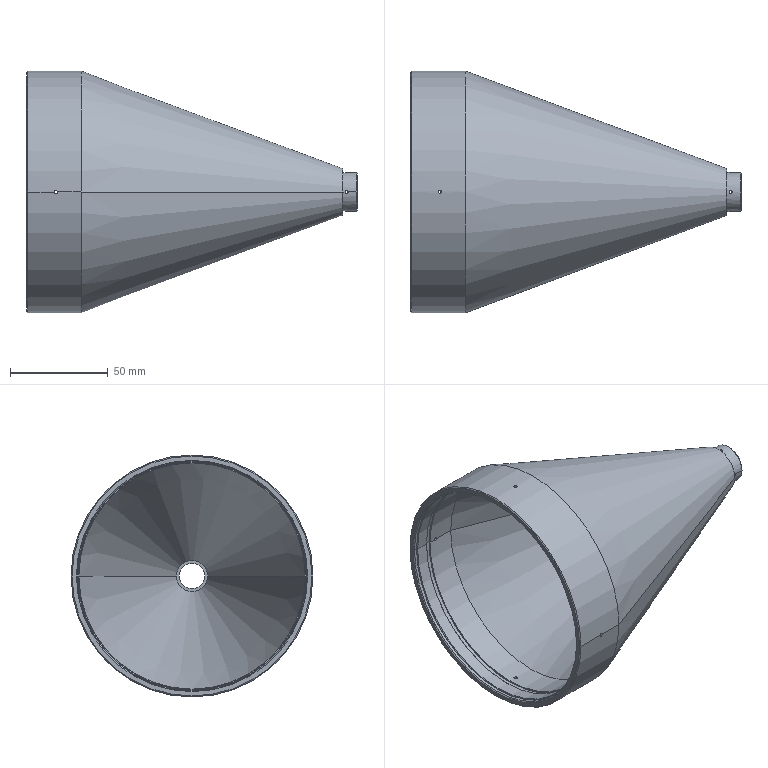Part | STEP file | lens barrel 2.stp.STEP-192.STEP | 1 solid | 64 faces | box 169.5 x 124 x 124 mm | volume 187714 mm3 | cylinder 36 | cone 18 | plane 10 | commonest cylinder face diameters 1.6 x16 117.5 x4 13 x2 15 x2 16 x2 17 x2